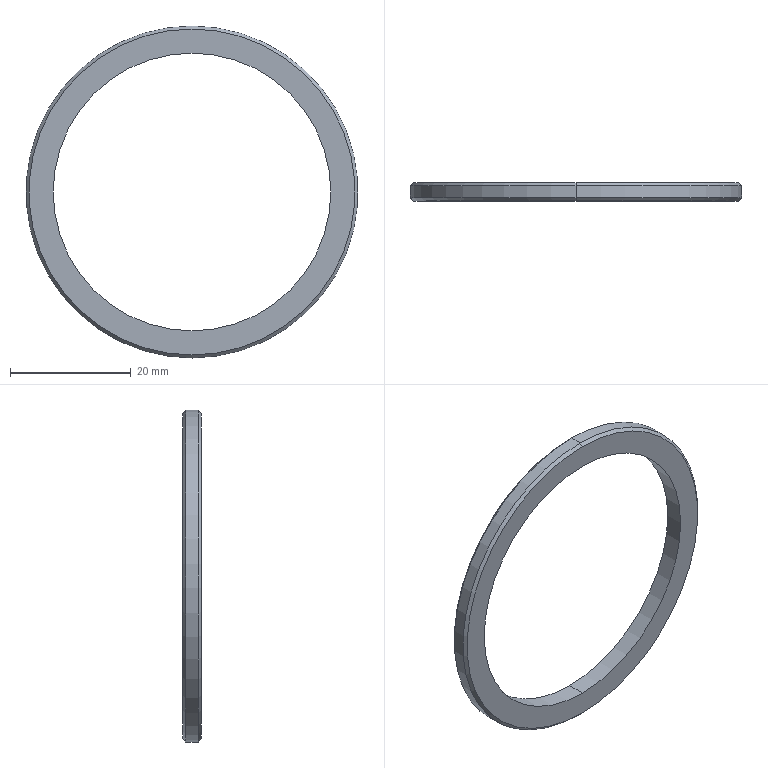Part | SolidWorks | features Chamfer 1, Extrusion 1 | 1 solid | 10 faces | box 55 x 3 x 55 mm | volume 2099 mm3 | cone 4 | cylinder 4 | plane 2 | commonest cylinder face diameters 46 x2 55 x2
STEP:
#1=CARTESIAN_POINT('',(0.,3.,27.));
#2=VERTEX_POINT('',#1);
#3=CARTESIAN_POINT('',(0.,3.,-27.));
#4=VERTEX_POINT('',#3);
#5=CARTESIAN_POINT('',(0.,3.,0.));
#6=DIRECTION('',(0.,1.,0.));
#7=DIRECTION('',(0.,0.,1.));
#8=AXIS2_PLACEMENT_3D('',#5,#6,#7);
#9=CIRCLE('',#8,27.);
#10=EDGE_CURVE('',#2,#4,#9,.T.);
#11=ORIENTED_EDGE('',*,*,#10,.F.);
#12=CARTESIAN_POINT('',(0.,2.5,27.5));
#13=VERTEX_POINT('',#12);
#14=CARTESIAN_POINT('',(0.,3.,27.));
#15=DIRECTION('',(0.,-0.7071,0.7071));
#16=VECTOR('',#15,1000.);
#17=LINE('',#14,#16);
#18=EDGE_CURVE('',#2,#13,#17,.T.);
#19=ORIENTED_EDGE('',*,*,#18,.T.);
#20=CARTESIAN_POINT('',(0.,2.5,-27.5));
#21=VERTEX_POINT('',#20);
#22=CARTESIAN_POINT('',(0.,2.5,0.));
#23=DIRECTION('',(0.,-1.,0.));
#24=DIRECTION('',(0.,0.,1.));
#25=AXIS2_PLACEMENT_3D('',#22,#23,#24);
#26=CIRCLE('',#25,27.5);
#27=EDGE_CURVE('',#21,#13,#26,.T.);
#28=ORIENTED_EDGE('',*,*,#27,.F.);
#29=CARTESIAN_POINT('',(0.,3.,-27.));
#30=DIRECTION('',(0.,-0.7071,-0.7071));
#31=VECTOR('',#30,1000.);
#32=LINE('',#29,#31);
#33=EDGE_CURVE('',#4,#21,#32,.T.);
#34=ORIENTED_EDGE('',*,*,#33,.F.);
#35=EDGE_LOOP('',(#11,#19,#28,#34));
#36=FACE_OUTER_BOUND('',#35,.T.);
#37=CARTESIAN_POINT('',(0.,3.,0.));
#38=DIRECTION('',(0.,-1.,0.));
#39=DIRECTION('',(0.,0.,-1.));
#40=AXIS2_PLACEMENT_3D('',#37,#38,#39);
#41=CONICAL_SURFACE('',#40,27.,0.7854);
#42=ADVANCED_FACE('',(#36),#41,.T.);
#43=CARTESIAN_POINT('',(0.,0.,-27.));
#44=VERTEX_POINT('',#43);
#45=CARTESIAN_POINT('',(0.,0.,27.));
#46=VERTEX_POINT('',#45);
#47=CARTESIAN_POINT('',(0.,0.,0.));
#48=DIRECTION('',(0.,-1.,0.));
#49=DIRECTION('',(0.,0.,1.));
#50=AXIS2_PLACEMENT_3D('',#47,#48,#49);
#51=CIRCLE('',#50,27.);
#52=EDGE_CURVE('',#44,#46,#51,.T.);
#53=ORIENTED_EDGE('',*,*,#52,.F.);
#54=CARTESIAN_POINT('',(0.,0.5,-27.5));
#55=VERTEX_POINT('',#54);
#56=CARTESIAN_POINT('',(0.,0.5,-27.5));
#57=DIRECTION('',(0.,0.7071,-0.7071));
#58=VECTOR('',#57,1000.);
#59=LINE('',#56,#58);
#60=EDGE_CURVE('',#44,#55,#59,.T.);
#61=ORIENTED_EDGE('',*,*,#60,.T.);
#62=CARTESIAN_POINT('',(0.,0.5,27.5));
#63=VERTEX_POINT('',#62);
#64=CARTESIAN_POINT('',(0.,0.5,0.));
#65=DIRECTION('',(0.,1.,0.));
#66=DIRECTION('',(0.,0.,1.));
#67=AXIS2_PLACEMENT_3D('',#64,#65,#66);
#68=CIRCLE('',#67,27.5);
#69=EDGE_CURVE('',#63,#55,#68,.T.);
#70=ORIENTED_EDGE('',*,*,#69,.F.);
#71=CARTESIAN_POINT('',(0.,0.5,27.5));
#72=DIRECTION('',(0.,0.7071,0.7071));
#73=VECTOR('',#72,1000.);
#74=LINE('',#71,#73);
#75=EDGE_CURVE('',#46,#63,#74,.T.);
#76=ORIENTED_EDGE('',*,*,#75,.F.);
#77=EDGE_LOOP('',(#53,#61,#70,#76));
#78=FACE_OUTER_BOUND('',#77,.T.);
#79=CARTESIAN_POINT('',(0.,0.5,0.));
#80=DIRECTION('',(0.,1.,0.));
#81=DIRECTION('',(0.,0.,1.));
#82=AXIS2_PLACEMENT_3D('',#79,#80,#81);
#83=CONICAL_SURFACE('',#82,27.5,0.7854);
#84=ADVANCED_FACE('',(#78),#83,.T.);
#85=CARTESIAN_POINT('',(0.,3.,-23.));
#86=VERTEX_POINT('',#85);
#87=CARTESIAN_POINT('',(0.,3.,23.));
#88=VERTEX_POINT('',#87);
#89=CARTESIAN_POINT('',(0.,3.,0.));
#90=DIRECTION('',(0.,1.,0.));
#91=DIRECTION('',(0.,0.,1.));
#92=AXIS2_PLACEMENT_3D('',#89,#90,#91);
#93=CIRCLE('',#92,23.);
#94=EDGE_CURVE('',#86,#88,#93,.T.);
#95=ORIENTED_EDGE('',*,*,#94,.T.);
#96=CARTESIAN_POINT('',(0.,0.,23.));
#97=VERTEX_POINT('',#96);
#98=CARTESIAN_POINT('',(0.,3.,23.));
#99=DIRECTION('',(0.,-1.,0.));
#100=VECTOR('',#99,1000.);
#101=LINE('',#98,#100);
#102=EDGE_CURVE('',#88,#97,#101,.T.);
#103=ORIENTED_EDGE('',*,*,#102,.T.);
#104=CARTESIAN_POINT('',(0.,0.,-23.));
#105=VERTEX_POINT('',#104);
#106=CARTESIAN_POINT('',(0.,0.,0.));
#107=DIRECTION('',(0.,1.,0.));
#108=DIRECTION('',(0.,0.,1.));
#109=AXIS2_PLACEMENT_3D('',#106,#107,#108);
#110=CIRCLE('',#109,23.);
#111=EDGE_CURVE('',#105,#97,#110,.T.);
#112=ORIENTED_EDGE('',*,*,#111,.F.);
#113=CARTESIAN_POINT('',(0.,3.,-23.));
#114=DIRECTION('',(0.,-1.,0.));
#115=VECTOR('',#114,1000.);
#116=LINE('',#113,#115);
#117=EDGE_CURVE('',#86,#105,#116,.T.);
#118=ORIENTED_EDGE('',*,*,#117,.F.);
#119=EDGE_LOOP('',(#95,#103,#112,#118));
#120=FACE_OUTER_BOUND('',#119,.T.);
#121=CARTESIAN_POINT('',(0.,3.,0.));
#122=DIRECTION('',(0.,-1.,0.));
#123=DIRECTION('',(0.,0.,-1.));
#124=AXIS2_PLACEMENT_3D('',#121,#122,#123);
#125=CYLINDRICAL_SURFACE('',#124,23.);
#126=ADVANCED_FACE('',(#120),#125,.F.);
#127=ORIENTED_EDGE('',*,*,#27,.T.);
#128=CARTESIAN_POINT('',(0.,3.,27.5));
#129=DIRECTION('',(0.,-1.,0.));
#130=VECTOR('',#129,1000.);
#131=LINE('',#128,#130);
#132=EDGE_CURVE('',#13,#63,#131,.T.);
#133=ORIENTED_EDGE('',*,*,#132,.T.);
#134=ORIENTED_EDGE('',*,*,#69,.T.);
#135=CARTESIAN_POINT('',(0.,3.,-27.5));
#136=DIRECTION('',(0.,-1.,0.));
#137=VECTOR('',#136,1000.);
#138=LINE('',#135,#137);
#139=EDGE_CURVE('',#21,#55,#138,.T.);
#140=ORIENTED_EDGE('',*,*,#139,.F.);
#141=EDGE_LOOP('',(#127,#133,#134,#140));
#142=FACE_OUTER_BOUND('',#141,.T.);
#143=CARTESIAN_POINT('',(0.,3.,0.));
#144=DIRECTION('',(0.,-1.,0.));
#145=DIRECTION('',(0.,0.,-1.));
#146=AXIS2_PLACEMENT_3D('',#143,#144,#145);
#147=CYLINDRICAL_SURFACE('',#146,27.5);
#148=ADVANCED_FACE('',(#142),#147,.T.);
#149=CARTESIAN_POINT('',(0.,3.,0.));
#150=DIRECTION('',(0.,1.,0.));
#151=DIRECTION('',(0.,0.,1.));
#152=AXIS2_PLACEMENT_3D('',#149,#150,#151);
#153=CIRCLE('',#152,27.);
#154=EDGE_CURVE('',#4,#2,#153,.T.);
#155=ORIENTED_EDGE('',*,*,#154,.T.);
#156=ORIENTED_EDGE('',*,*,#10,.T.);
#157=EDGE_LOOP('',(#155,#156));
#158=FACE_OUTER_BOUND('',#157,.T.);
#159=ORIENTED_EDGE('',*,*,#94,.F.);
#160=CARTESIAN_POINT('',(0.,3.,0.));
#161=DIRECTION('',(0.,1.,0.));
#162=DIRECTION('',(0.,0.,1.));
#163=AXIS2_PLACEMENT_3D('',#160,#161,#162);
#164=CIRCLE('',#163,23.);
#165=EDGE_CURVE('',#88,#86,#164,.T.);
#166=ORIENTED_EDGE('',*,*,#165,.F.);
#167=EDGE_LOOP('',(#159,#166));
#168=FACE_BOUND('',#167,.T.);
#169=CARTESIAN_POINT('',(0.,3.,0.));
#170=DIRECTION('',(0.,1.,0.));
#171=DIRECTION('',(0.,0.,1.));
#172=AXIS2_PLACEMENT_3D('',#169,#170,#171);
#173=PLANE('',#172);
#174=ADVANCED_FACE('',(#158,#168),#173,.T.);
#175=CARTESIAN_POINT('',(0.,0.,0.));
#176=DIRECTION('',(0.,-1.,0.));
#177=DIRECTION('',(0.,0.,1.));
#178=AXIS2_PLACEMENT_3D('',#175,#176,#177);
#179=CIRCLE('',#178,27.);
#180=EDGE_CURVE('',#46,#44,#179,.T.);
#181=ORIENTED_EDGE('',*,*,#180,.T.);
#182=ORIENTED_EDGE('',*,*,#52,.T.);
#183=EDGE_LOOP('',(#181,#182));
#184=FACE_OUTER_BOUND('',#183,.T.);
#185=ORIENTED_EDGE('',*,*,#111,.T.);
#186=CARTESIAN_POINT('',(0.,0.,0.));
#187=DIRECTION('',(0.,1.,0.));
#188=DIRECTION('',(0.,0.,1.));
#189=AXIS2_PLACEMENT_3D('',#186,#187,#188);
#190=CIRCLE('',#189,23.);
#191=EDGE_CURVE('',#97,#105,#190,.T.);
#192=ORIENTED_EDGE('',*,*,#191,.T.);
#193=EDGE_LOOP('',(#185,#192));
#194=FACE_BOUND('',#193,.T.);
#195=CARTESIAN_POINT('',(0.,0.,0.));
#196=DIRECTION('',(0.,1.,0.));
#197=DIRECTION('',(0.,0.,1.));
#198=AXIS2_PLACEMENT_3D('',#195,#196,#197);
#199=PLANE('',#198);
#200=ADVANCED_FACE('',(#184,#194),#199,.F.);
#201=ORIENTED_EDGE('',*,*,#132,.F.);
#202=CARTESIAN_POINT('',(0.,2.5,0.));
#203=DIRECTION('',(0.,-1.,0.));
#204=DIRECTION('',(0.,0.,1.));
#205=AXIS2_PLACEMENT_3D('',#202,#203,#204);
#206=CIRCLE('',#205,27.5);
#207=EDGE_CURVE('',#13,#21,#206,.T.);
#208=ORIENTED_EDGE('',*,*,#207,.T.);
#209=ORIENTED_EDGE('',*,*,#139,.T.);
#210=CARTESIAN_POINT('',(0.,0.5,0.));
#211=DIRECTION('',(0.,1.,0.));
#212=DIRECTION('',(0.,0.,1.));
#213=AXIS2_PLACEMENT_3D('',#210,#211,#212);
#214=CIRCLE('',#213,27.5);
#215=EDGE_CURVE('',#55,#63,#214,.T.);
#216=ORIENTED_EDGE('',*,*,#215,.T.);
#217=EDGE_LOOP('',(#201,#208,#209,#216));
#218=FACE_OUTER_BOUND('',#217,.T.);
#219=CARTESIAN_POINT('',(0.,3.,0.));
#220=DIRECTION('',(0.,-1.,0.));
#221=DIRECTION('',(0.,0.,-1.));
#222=AXIS2_PLACEMENT_3D('',#219,#220,#221);
#223=CYLINDRICAL_SURFACE('',#222,27.5);
#224=ADVANCED_FACE('',(#218),#223,.T.);
#225=ORIENTED_EDGE('',*,*,#102,.F.);
#226=ORIENTED_EDGE('',*,*,#165,.T.);
#227=ORIENTED_EDGE('',*,*,#117,.T.);
#228=ORIENTED_EDGE('',*,*,#191,.F.);
#229=EDGE_LOOP('',(#225,#226,#227,#228));
#230=FACE_OUTER_BOUND('',#229,.T.);
#231=CARTESIAN_POINT('',(0.,3.,0.));
#232=DIRECTION('',(0.,-1.,0.));
#233=DIRECTION('',(0.,0.,-1.));
#234=AXIS2_PLACEMENT_3D('',#231,#232,#233);
#235=CYLINDRICAL_SURFACE('',#234,23.);
#236=ADVANCED_FACE('',(#230),#235,.F.);
#237=ORIENTED_EDGE('',*,*,#60,.F.);
#238=ORIENTED_EDGE('',*,*,#180,.F.);
#239=ORIENTED_EDGE('',*,*,#75,.T.);
#240=ORIENTED_EDGE('',*,*,#215,.F.);
#241=EDGE_LOOP('',(#237,#238,#239,#240));
#242=FACE_OUTER_BOUND('',#241,.T.);
#243=CARTESIAN_POINT('',(0.,0.5,0.));
#244=DIRECTION('',(0.,1.,0.));
#245=DIRECTION('',(0.,0.,1.));
#246=AXIS2_PLACEMENT_3D('',#243,#244,#245);
#247=CONICAL_SURFACE('',#246,27.5,0.7854);
#248=ADVANCED_FACE('',(#242),#247,.T.);
#249=ORIENTED_EDGE('',*,*,#18,.F.);
#250=ORIENTED_EDGE('',*,*,#154,.F.);
#251=ORIENTED_EDGE('',*,*,#33,.T.);
#252=ORIENTED_EDGE('',*,*,#207,.F.);
#253=EDGE_LOOP('',(#249,#250,#251,#252));
#254=FACE_OUTER_BOUND('',#253,.T.);
#255=CARTESIAN_POINT('',(0.,3.,0.));
#256=DIRECTION('',(0.,-1.,0.));
#257=DIRECTION('',(0.,0.,-1.));
#258=AXIS2_PLACEMENT_3D('',#255,#256,#257);
#259=CONICAL_SURFACE('',#258,27.,0.7854);
#260=ADVANCED_FACE('',(#254),#259,.T.);
#261=CLOSED_SHELL('',(#42,#84,#126,#148,#174,#200,#224,#236,#248,#260));
#262=MANIFOLD_SOLID_BREP('',#261);
#263=CARTESIAN_POINT('',(0.,0.,0.));
#264=DIRECTION('',(0.,0.,1.));
#265=DIRECTION('',(1.,0.,0.));
#266=AXIS2_PLACEMENT_3D('',#263,#264,#265);
#267=(LENGTH_UNIT()NAMED_UNIT(*)SI_UNIT(.MILLI.,.METRE.));
#268=UNCERTAINTY_MEASURE_WITH_UNIT(LENGTH_MEASURE(0.00001),#267,'','');
#269=(NAMED_UNIT(*)PLANE_ANGLE_UNIT()SI_UNIT($,.RADIAN.));
#270=(NAMED_UNIT(*)SI_UNIT($,.STERADIAN.)SOLID_ANGLE_UNIT());
#271=(GEOMETRIC_REPRESENTATION_CONTEXT(3)GLOBAL_UNCERTAINTY_ASSIGNED_CONTEXT((#268))GLOBAL_UNIT_ASSIGNED_CONTEXT((#267,#269,#270))REPRESENTATION_CONTEXT('',''));
#272=ADVANCED_BREP_SHAPE_REPRESENTATION('',(#262,#266),#271);